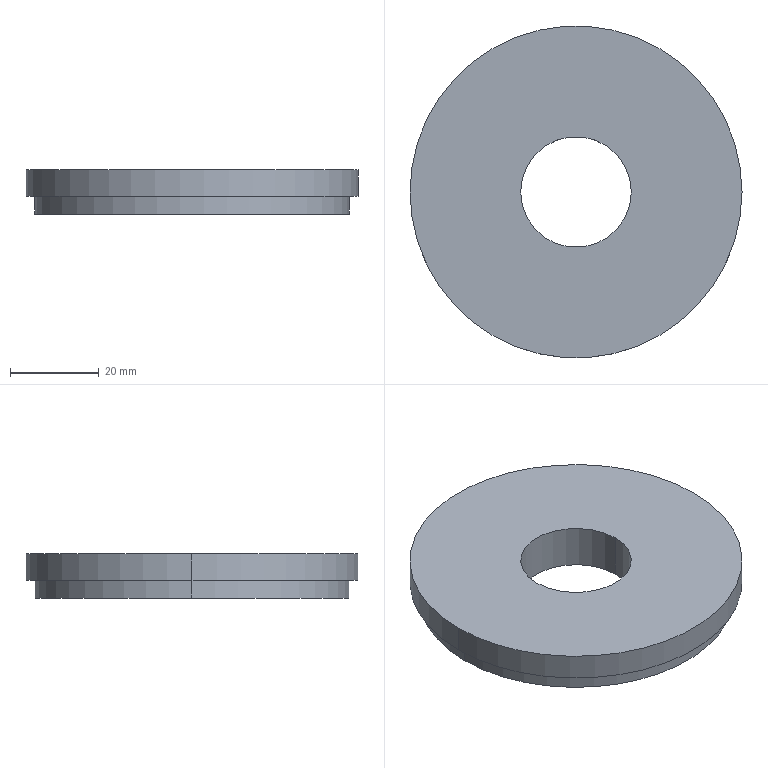Part | STEP file | Microwave Drying Flat Conveyor-CN2500x400-107-103 | 1 solid | 9 faces | box 75 x 75 x 10 mm | volume 37435 mm3 | cylinder 6 | plane 3 | commonest cylinder face diameters 25 x2 71 x2 75 x2
STEP:
#1=CARTESIAN_POINT('',(-12.5,0.,-10.));
#2=VERTEX_POINT('',#1);
#3=CARTESIAN_POINT('',(12.5,0.,-10.));
#4=VERTEX_POINT('',#3);
#5=CARTESIAN_POINT('',(0.,0.,-10.));
#6=DIRECTION('',(0.,0.,1.));
#7=DIRECTION('',(1.,0.,0.));
#8=AXIS2_PLACEMENT_3D('',#5,#6,#7);
#9=CIRCLE('',#8,12.5);
#10=EDGE_CURVE('',#2,#4,#9,.T.);
#11=ORIENTED_EDGE('',*,*,#10,.F.);
#12=CARTESIAN_POINT('',(-12.5,0.,0.));
#13=VERTEX_POINT('',#12);
#14=CARTESIAN_POINT('',(-12.5,0.,0.));
#15=DIRECTION('',(0.,0.,1.));
#16=VECTOR('',#15,1000.);
#17=LINE('',#14,#16);
#18=EDGE_CURVE('',#2,#13,#17,.T.);
#19=ORIENTED_EDGE('',*,*,#18,.T.);
#20=CARTESIAN_POINT('',(12.5,0.,0.));
#21=VERTEX_POINT('',#20);
#22=CARTESIAN_POINT('',(0.,0.,0.));
#23=DIRECTION('',(0.,0.,1.));
#24=DIRECTION('',(1.,0.,0.));
#25=AXIS2_PLACEMENT_3D('',#22,#23,#24);
#26=CIRCLE('',#25,12.5);
#27=EDGE_CURVE('',#13,#21,#26,.T.);
#28=ORIENTED_EDGE('',*,*,#27,.T.);
#29=CARTESIAN_POINT('',(12.5,0.,0.));
#30=DIRECTION('',(0.,0.,1.));
#31=VECTOR('',#30,1000.);
#32=LINE('',#29,#31);
#33=EDGE_CURVE('',#4,#21,#32,.T.);
#34=ORIENTED_EDGE('',*,*,#33,.F.);
#35=EDGE_LOOP('',(#11,#19,#28,#34));
#36=FACE_OUTER_BOUND('',#35,.T.);
#37=CARTESIAN_POINT('',(0.,0.,0.));
#38=DIRECTION('',(0.,0.,1.));
#39=DIRECTION('',(1.,0.,0.));
#40=AXIS2_PLACEMENT_3D('',#37,#38,#39);
#41=CYLINDRICAL_SURFACE('',#40,12.5);
#42=ADVANCED_FACE('',(#36),#41,.F.);
#43=CARTESIAN_POINT('',(35.5,0.,-10.));
#44=VERTEX_POINT('',#43);
#45=CARTESIAN_POINT('',(-35.5,0.,-10.));
#46=VERTEX_POINT('',#45);
#47=CARTESIAN_POINT('',(0.,0.,-10.));
#48=DIRECTION('',(0.,0.,1.));
#49=DIRECTION('',(1.,0.,0.));
#50=AXIS2_PLACEMENT_3D('',#47,#48,#49);
#51=CIRCLE('',#50,35.5);
#52=EDGE_CURVE('',#44,#46,#51,.T.);
#53=ORIENTED_EDGE('',*,*,#52,.T.);
#54=CARTESIAN_POINT('',(-35.5,0.,-6.));
#55=VERTEX_POINT('',#54);
#56=CARTESIAN_POINT('',(-35.5,0.,0.));
#57=DIRECTION('',(0.,0.,1.));
#58=VECTOR('',#57,1000.);
#59=LINE('',#56,#58);
#60=EDGE_CURVE('',#46,#55,#59,.T.);
#61=ORIENTED_EDGE('',*,*,#60,.T.);
#62=CARTESIAN_POINT('',(35.5,0.,-6.));
#63=VERTEX_POINT('',#62);
#64=CARTESIAN_POINT('',(0.,0.,-6.));
#65=DIRECTION('',(0.,0.,1.));
#66=DIRECTION('',(1.,0.,0.));
#67=AXIS2_PLACEMENT_3D('',#64,#65,#66);
#68=CIRCLE('',#67,35.5);
#69=EDGE_CURVE('',#63,#55,#68,.T.);
#70=ORIENTED_EDGE('',*,*,#69,.F.);
#71=CARTESIAN_POINT('',(35.5,0.,0.));
#72=DIRECTION('',(0.,0.,1.));
#73=VECTOR('',#72,1000.);
#74=LINE('',#71,#73);
#75=EDGE_CURVE('',#44,#63,#74,.T.);
#76=ORIENTED_EDGE('',*,*,#75,.F.);
#77=EDGE_LOOP('',(#53,#61,#70,#76));
#78=FACE_OUTER_BOUND('',#77,.T.);
#79=CARTESIAN_POINT('',(0.,0.,0.));
#80=DIRECTION('',(0.,0.,1.));
#81=DIRECTION('',(1.,0.,0.));
#82=AXIS2_PLACEMENT_3D('',#79,#80,#81);
#83=CYLINDRICAL_SURFACE('',#82,35.5);
#84=ADVANCED_FACE('',(#78),#83,.T.);
#85=CARTESIAN_POINT('',(37.5,0.,-6.));
#86=VERTEX_POINT('',#85);
#87=CARTESIAN_POINT('',(-37.5,0.,-6.));
#88=VERTEX_POINT('',#87);
#89=CARTESIAN_POINT('',(0.,0.,-6.));
#90=DIRECTION('',(0.,0.,1.));
#91=DIRECTION('',(1.,0.,0.));
#92=AXIS2_PLACEMENT_3D('',#89,#90,#91);
#93=CIRCLE('',#92,37.5);
#94=EDGE_CURVE('',#86,#88,#93,.T.);
#95=ORIENTED_EDGE('',*,*,#94,.T.);
#96=CARTESIAN_POINT('',(-37.5,0.,0.));
#97=VERTEX_POINT('',#96);
#98=CARTESIAN_POINT('',(-37.5,0.,0.));
#99=DIRECTION('',(0.,0.,1.));
#100=VECTOR('',#99,1000.);
#101=LINE('',#98,#100);
#102=EDGE_CURVE('',#88,#97,#101,.T.);
#103=ORIENTED_EDGE('',*,*,#102,.T.);
#104=CARTESIAN_POINT('',(37.5,0.,0.));
#105=VERTEX_POINT('',#104);
#106=CARTESIAN_POINT('',(0.,0.,0.));
#107=DIRECTION('',(0.,0.,1.));
#108=DIRECTION('',(1.,0.,0.));
#109=AXIS2_PLACEMENT_3D('',#106,#107,#108);
#110=CIRCLE('',#109,37.5);
#111=EDGE_CURVE('',#105,#97,#110,.T.);
#112=ORIENTED_EDGE('',*,*,#111,.F.);
#113=CARTESIAN_POINT('',(37.5,0.,0.));
#114=DIRECTION('',(0.,0.,1.));
#115=VECTOR('',#114,1000.);
#116=LINE('',#113,#115);
#117=EDGE_CURVE('',#86,#105,#116,.T.);
#118=ORIENTED_EDGE('',*,*,#117,.F.);
#119=EDGE_LOOP('',(#95,#103,#112,#118));
#120=FACE_OUTER_BOUND('',#119,.T.);
#121=CARTESIAN_POINT('',(0.,0.,0.));
#122=DIRECTION('',(0.,0.,1.));
#123=DIRECTION('',(1.,0.,0.));
#124=AXIS2_PLACEMENT_3D('',#121,#122,#123);
#125=CYLINDRICAL_SURFACE('',#124,37.5);
#126=ADVANCED_FACE('',(#120),#125,.T.);
#127=ORIENTED_EDGE('',*,*,#102,.F.);
#128=CARTESIAN_POINT('',(0.,0.,-6.));
#129=DIRECTION('',(0.,0.,1.));
#130=DIRECTION('',(1.,0.,0.));
#131=AXIS2_PLACEMENT_3D('',#128,#129,#130);
#132=CIRCLE('',#131,37.5);
#133=EDGE_CURVE('',#88,#86,#132,.T.);
#134=ORIENTED_EDGE('',*,*,#133,.T.);
#135=ORIENTED_EDGE('',*,*,#117,.T.);
#136=CARTESIAN_POINT('',(0.,0.,0.));
#137=DIRECTION('',(0.,0.,1.));
#138=DIRECTION('',(1.,0.,0.));
#139=AXIS2_PLACEMENT_3D('',#136,#137,#138);
#140=CIRCLE('',#139,37.5);
#141=EDGE_CURVE('',#97,#105,#140,.T.);
#142=ORIENTED_EDGE('',*,*,#141,.F.);
#143=EDGE_LOOP('',(#127,#134,#135,#142));
#144=FACE_OUTER_BOUND('',#143,.T.);
#145=CARTESIAN_POINT('',(0.,0.,0.));
#146=DIRECTION('',(0.,0.,1.));
#147=DIRECTION('',(1.,0.,0.));
#148=AXIS2_PLACEMENT_3D('',#145,#146,#147);
#149=CYLINDRICAL_SURFACE('',#148,37.5);
#150=ADVANCED_FACE('',(#144),#149,.T.);
#151=ORIENTED_EDGE('',*,*,#94,.F.);
#152=ORIENTED_EDGE('',*,*,#133,.F.);
#153=EDGE_LOOP('',(#151,#152));
#154=FACE_OUTER_BOUND('',#153,.T.);
#155=ORIENTED_EDGE('',*,*,#69,.T.);
#156=CARTESIAN_POINT('',(0.,0.,-6.));
#157=DIRECTION('',(0.,0.,1.));
#158=DIRECTION('',(1.,0.,0.));
#159=AXIS2_PLACEMENT_3D('',#156,#157,#158);
#160=CIRCLE('',#159,35.5);
#161=EDGE_CURVE('',#55,#63,#160,.T.);
#162=ORIENTED_EDGE('',*,*,#161,.T.);
#163=EDGE_LOOP('',(#155,#162));
#164=FACE_BOUND('',#163,.T.);
#165=CARTESIAN_POINT('',(0.,37.5,-6.));
#166=DIRECTION('',(0.,0.,1.));
#167=DIRECTION('',(1.,0.,0.));
#168=AXIS2_PLACEMENT_3D('',#165,#166,#167);
#169=PLANE('',#168);
#170=ADVANCED_FACE('',(#154,#164),#169,.F.);
#171=ORIENTED_EDGE('',*,*,#60,.F.);
#172=CARTESIAN_POINT('',(0.,0.,-10.));
#173=DIRECTION('',(0.,0.,1.));
#174=DIRECTION('',(1.,0.,0.));
#175=AXIS2_PLACEMENT_3D('',#172,#173,#174);
#176=CIRCLE('',#175,35.5);
#177=EDGE_CURVE('',#46,#44,#176,.T.);
#178=ORIENTED_EDGE('',*,*,#177,.T.);
#179=ORIENTED_EDGE('',*,*,#75,.T.);
#180=ORIENTED_EDGE('',*,*,#161,.F.);
#181=EDGE_LOOP('',(#171,#178,#179,#180));
#182=FACE_OUTER_BOUND('',#181,.T.);
#183=CARTESIAN_POINT('',(0.,0.,0.));
#184=DIRECTION('',(0.,0.,1.));
#185=DIRECTION('',(1.,0.,0.));
#186=AXIS2_PLACEMENT_3D('',#183,#184,#185);
#187=CYLINDRICAL_SURFACE('',#186,35.5);
#188=ADVANCED_FACE('',(#182),#187,.T.);
#189=ORIENTED_EDGE('',*,*,#52,.F.);
#190=ORIENTED_EDGE('',*,*,#177,.F.);
#191=EDGE_LOOP('',(#189,#190));
#192=FACE_OUTER_BOUND('',#191,.T.);
#193=CARTESIAN_POINT('',(0.,0.,-10.));
#194=DIRECTION('',(0.,0.,1.));
#195=DIRECTION('',(1.,0.,0.));
#196=AXIS2_PLACEMENT_3D('',#193,#194,#195);
#197=CIRCLE('',#196,12.5);
#198=EDGE_CURVE('',#4,#2,#197,.T.);
#199=ORIENTED_EDGE('',*,*,#198,.T.);
#200=ORIENTED_EDGE('',*,*,#10,.T.);
#201=EDGE_LOOP('',(#199,#200));
#202=FACE_BOUND('',#201,.T.);
#203=CARTESIAN_POINT('',(0.,35.5,-10.));
#204=DIRECTION('',(0.,0.,1.));
#205=DIRECTION('',(1.,0.,0.));
#206=AXIS2_PLACEMENT_3D('',#203,#204,#205);
#207=PLANE('',#206);
#208=ADVANCED_FACE('',(#192,#202),#207,.F.);
#209=ORIENTED_EDGE('',*,*,#18,.F.);
#210=ORIENTED_EDGE('',*,*,#198,.F.);
#211=ORIENTED_EDGE('',*,*,#33,.T.);
#212=CARTESIAN_POINT('',(0.,0.,0.));
#213=DIRECTION('',(0.,0.,1.));
#214=DIRECTION('',(1.,0.,0.));
#215=AXIS2_PLACEMENT_3D('',#212,#213,#214);
#216=CIRCLE('',#215,12.5);
#217=EDGE_CURVE('',#21,#13,#216,.T.);
#218=ORIENTED_EDGE('',*,*,#217,.T.);
#219=EDGE_LOOP('',(#209,#210,#211,#218));
#220=FACE_OUTER_BOUND('',#219,.T.);
#221=CARTESIAN_POINT('',(0.,0.,0.));
#222=DIRECTION('',(0.,0.,1.));
#223=DIRECTION('',(1.,0.,0.));
#224=AXIS2_PLACEMENT_3D('',#221,#222,#223);
#225=CYLINDRICAL_SURFACE('',#224,12.5);
#226=ADVANCED_FACE('',(#220),#225,.F.);
#227=ORIENTED_EDGE('',*,*,#217,.F.);
#228=ORIENTED_EDGE('',*,*,#27,.F.);
#229=EDGE_LOOP('',(#227,#228));
#230=FACE_BOUND('',#229,.T.);
#231=ORIENTED_EDGE('',*,*,#111,.T.);
#232=ORIENTED_EDGE('',*,*,#141,.T.);
#233=EDGE_LOOP('',(#231,#232));
#234=FACE_OUTER_BOUND('',#233,.T.);
#235=CARTESIAN_POINT('',(0.,12.5,0.));
#236=DIRECTION('',(0.,0.,-1.));
#237=DIRECTION('',(-1.,0.,0.));
#238=AXIS2_PLACEMENT_3D('',#235,#236,#237);
#239=PLANE('',#238);
#240=ADVANCED_FACE('',(#230,#234),#239,.F.);
#241=CLOSED_SHELL('',(#42,#84,#126,#150,#170,#188,#208,#226,#240));
#242=MANIFOLD_SOLID_BREP('',#241);
#243=CARTESIAN_POINT('',(0.,0.,0.));
#244=DIRECTION('',(0.,0.,1.));
#245=DIRECTION('',(1.,0.,0.));
#246=AXIS2_PLACEMENT_3D('',#243,#244,#245);
#247=(LENGTH_UNIT()NAMED_UNIT(*)SI_UNIT(.MILLI.,.METRE.));
#248=UNCERTAINTY_MEASURE_WITH_UNIT(LENGTH_MEASURE(0.00001),#247,'','');
#249=(NAMED_UNIT(*)PLANE_ANGLE_UNIT()SI_UNIT($,.RADIAN.));
#250=(NAMED_UNIT(*)SI_UNIT($,.STERADIAN.)SOLID_ANGLE_UNIT());
#251=(GEOMETRIC_REPRESENTATION_CONTEXT(3)GLOBAL_UNCERTAINTY_ASSIGNED_CONTEXT((#248))GLOBAL_UNIT_ASSIGNED_CONTEXT((#247,#249,#250))REPRESENTATION_CONTEXT('',''));
#252=ADVANCED_BREP_SHAPE_REPRESENTATION('',(#242,#246),#251);